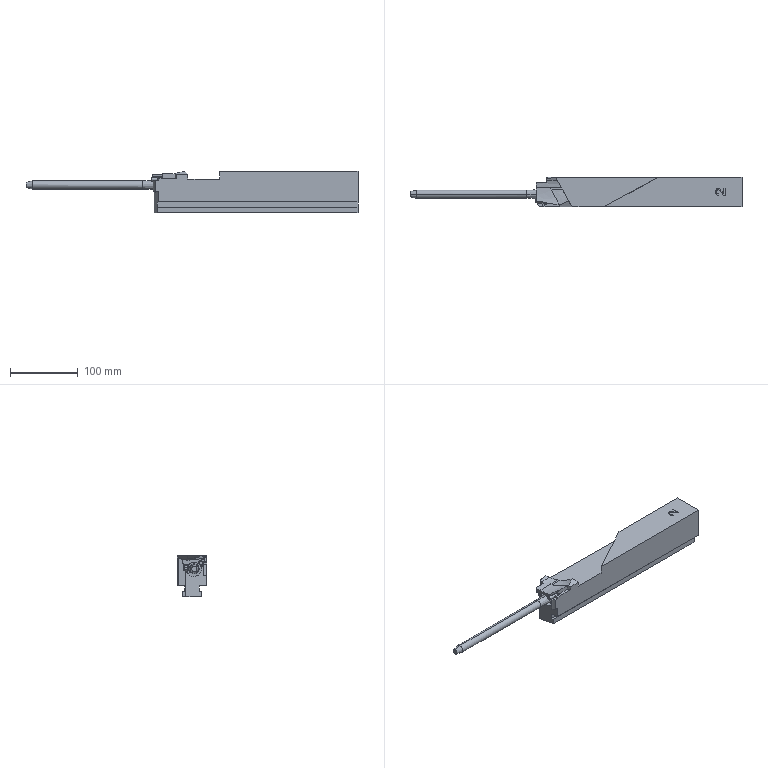Part | Creo | 1 solid | 87 faces | box 489.135 x 44.017 x 61.2 mm | volume 664373 mm3 | plane 47 | cylinder 15 | spline 10 | other 8 | cone 7 | commonest cylinder face diameters 4.02 x3 5.025 x2 12 x2 40.216 x2 5.276 x1 12.06 x1